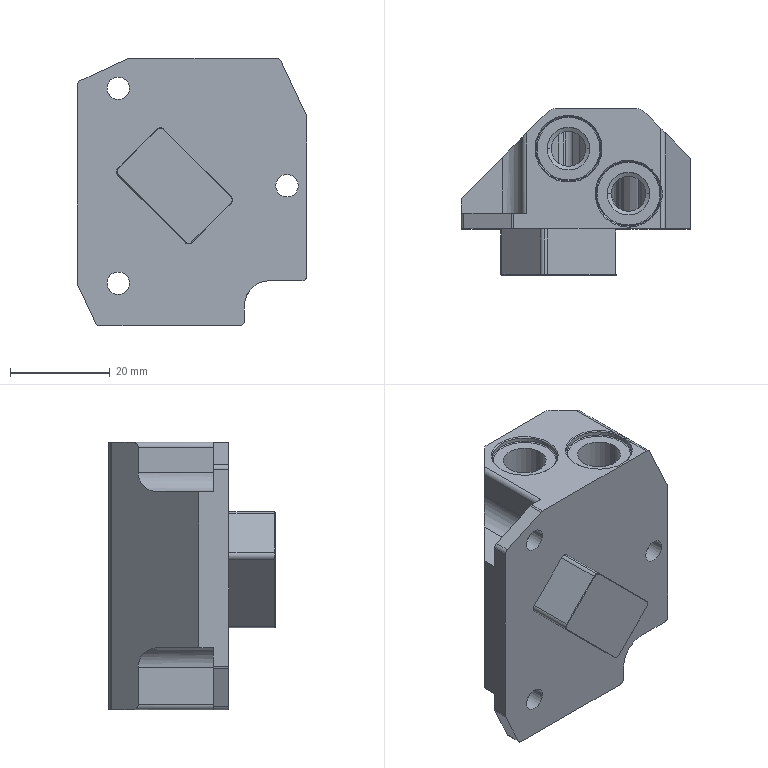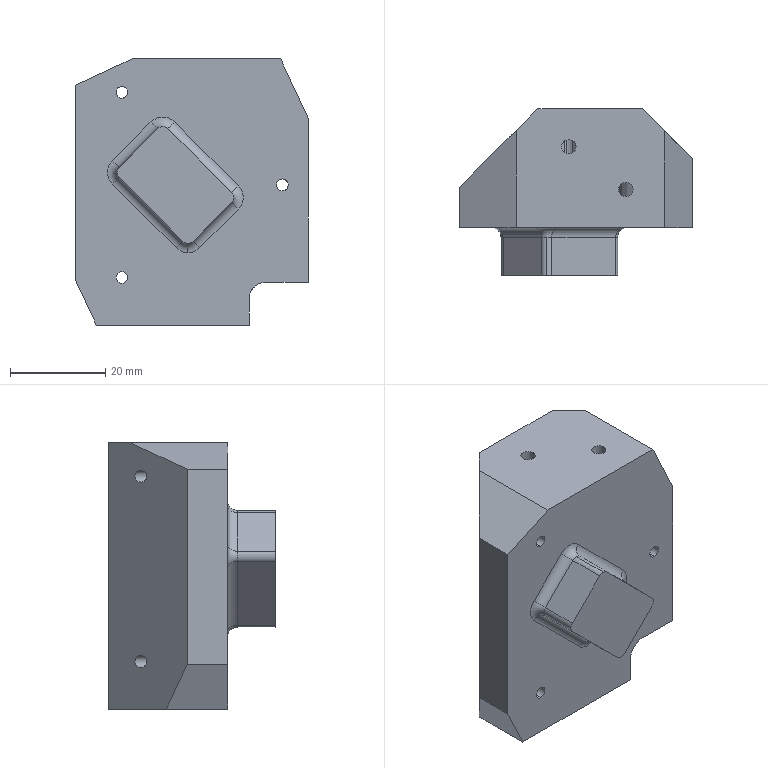CAM job | NX | 3+2 milling, 5-axis milling, drilling | part box 46 x 33.25 x 53.5 mm | stock box 49 x 35 x 56 mm
Tools:
number,name,description,diameter,corner_radius,flute_length,length,flutes
10,D3R0.2,Milling Tool-5 Parameters,3.0,0.2,50.0,75.0,2
0,D6R0.5,Milling Tool-5 Parameters,6.0,0.5,50.0,75.0,2
7,D3-9-D4-50-3T-ROUGH,D3-9-D4-50-3T,3.0,0.2,9.0,10.0,3
3,D5-15-D6-50-3T-ROUGH,D5-15-D6-50-3T,5.0,0.0,15.0,16.0,3
2,D10-30-D10-75-3T-ROUGH,D10-30-D10-75-3T-粗,10.0,0.0,30.0,75.0,2
5,D10-30-D10-75-3T-FINISH,D10-30-D10-75-3T,10.0,0.0,30.0,75.0,3
0,D63面刀,D63面刀,63.0,0.0,30.0,30.0,4
8,倒角D4-90度,倒角D4-90度,4.0,0.0,5.0,50.0,2
6,球刀R2-8-D4-50,球刀R2-8-D4-50,4.0,2.0,8.0,50.0,2
9,G8-1,Thread Mill,7.7,0.0,10.0,50.0,2
Operations:
program,operation,operation_type,tool,method,geometry_group,spindle_rpm,surface_speed,feed_per_tooth,feed_cut,feed_plunge,cut_length_mm,path_length_mm,cut_time_min,machine_time_min
NONE,PLANAR_MILL_6,PlanarMilling,D3-9-D4-50-3T-ROUGH,METHOD,C-G56,4500.0,70.0,0.0222,300.0,100.0,533.407,618.291,1.778,1.786
NONE,PLANAR_MILL_6_COPY,PlanarMilling,D3-9-D4-50-3T-ROUGH,METHOD,C-G56,4500.0,70.0,0.0222,300.0,100.0,93.82,186.111,0.3127,0.322
A1,PLANAR_MILL,PlanarMilling,D63面刀,METHOD,A-G54,3500.0,549.0,0.0571,800.0,100.0,126.5,182.5,0.1581,0.1637
A2,动态粗,CavityMilling,D10-30-D10-75-3T-ROUGH,METHOD,WORKPIECE_54,5500.0,172.0,0.1364,1500.0,100.0,5347.991,8574.346,3.44,3.763
A2,动态粗_COPY,CavityMilling,D5-15-D6-50-3T-ROUGH,METHOD,WORKPIECE_54,5500.0,86.0,0.0909,1500.0,100.0,1437.357,2628.154,0.9386,1.058
A3,CURVE_DRIVE,SurfaceContour,D6R0.5,METHOD,A-G54,5500.0,103.0,0.2727,3000.0,100.0,31035.578,31231.563,10.345,10.365
A4,PLANAR_MILL_1,PlanarMilling,D10-30-D10-75-3T-FINISH,METHOD,A-G54,4000.0,100.0,0.1178,800.0,100.0,453.139,559.139,0.5664,0.577
A4,PLANAR_MILL_2_COPY_1,PlanarMilling,D5-15-D6-50-3T-ROUGH,METHOD,A-G54,4500.0,70.0,0.0593,800.0,100.0,592.101,1419.752,0.7401,0.8229
A4,PLANAR_MILL_2,PlanarMilling,D5-15-D6-50-3T-ROUGH,METHOD,A-G54,4500.0,70.0,0.0593,800.0,100.0,190.71,630.914,0.2384,0.2824
A4,PLANAR_MILL_2_COPY,PlanarMilling,D5-15-D6-50-3T-ROUGH,METHOD,A-G54,4500.0,70.0,0.0593,800.0,100.0,288.693,485.736,0.3609,0.3806
A5,3_AXIS_DEBURRING,TpMultiAxisDeburring,球刀R2-8-D4-50,METHOD,A-G54,3500.0,43.0,0.1143,800.0,90.0,298.577,728.612,0.3745,0.3745
A6,PLANAR_MILL_COPY,PlanarMilling,D63面刀,METHOD,A-G54,3500.0,692.0,0.0286,400.0,100.0,126.5,182.52,0.3163,0.3219
B1,FLOOR_FACING,VolumeBased25DMillingOperation,D10-30-D10-75-3T-ROUGH,METHOD,B-G55,3500.0,109.0,0.1429,1000.0,100.0,84.508,124.308,0.0845,0.0885
B1,PLANAR_MILL_5_COPY,PlanarMilling,D10-30-D10-75-3T-ROUGH,METHOD,B-G55,3500.0,109.0,0.1429,1000.0,100.0,560.846,594.846,0.5608,0.5642
B1,HOLE_MILLING,CylinderMilling,D3-9-D4-50-3T-ROUGH,METHOD,B-G55,3000.0,28.0,0.0444,400.0,100.0,257.302,464.245,0.6433,0.6639
B1,FLOOR_FACING_1,VolumeBased25DMillingOperation,D10-30-D10-75-3T-FINISH,METHOD,B-G55,3500.0,109.0,0.0571,600.0,100.0,80.24,120.24,0.1337,0.1377
B1,PLANAR_MILL_5,PlanarMilling,D10-30-D10-75-3T-FINISH,METHOD,B-G55,3500.0,109.0,0.0571,600.0,100.0,561.135,595.135,0.9352,0.9386
B1,PLANAR_MILL_3,PlanarMilling,D10-30-D10-75-3T-FINISH,METHOD,B-G55,3500.0,109.0,0.0571,600.0,100.0,107.982,162.472,0.18,0.1854
B1,PLANAR_MILL_3_COPY,PlanarMilling,倒角D4-90度,METHOD,B-G55,3500.0,43.0,0.1429,1000.0,100.0,85.96,124.95,0.086,0.0899
B1,PLANAR_MILL_3_COPY_COPY,PlanarMilling,倒角D4-90度,METHOD,B-G55,3500.0,43.0,0.1429,1000.0,100.0,204.182,243.172,0.2042,0.2081
B1,PLANAR_MILL_3_COPY_COPY_1,PlanarMilling,倒角D4-90度,METHOD,B-G55,3500.0,43.0,0.1429,1000.0,100.0,28.34,223.655,0.0283,0.0479
C1,PLANAR_MILL_7,PlanarMilling,D5-15-D6-50-3T-ROUGH,METHOD,C-G56,4500.0,70.0,0.0222,300.0,100.0,543.659,650.337,1.812,1.823
C1,PLANAR_MILL_7_COPY_1,PlanarMilling,D5-15-D6-50-3T-ROUGH,METHOD,C-G56,4500.0,70.0,0.0222,300.0,100.0,215.142,343.432,0.7171,0.73
C1,PLANAR_MILL_4,PlanarMilling,D3R0.2,METHOD,C-G56,4500.0,42.0,0.0667,600.0,100.0,545.494,630.942,0.9092,0.9177
C1,PLANAR_MILL_4_COPY,PlanarMilling,D3R0.2,METHOD,C-G56,4500.0,42.0,0.0667,300.0,100.0,89.226,182.033,0.2974,0.3067
C1,PLANAR_MILL_7_COPY_COPY,PlanarMilling,倒角D4-90度,METHOD,C-G56,3000.0,37.0,0.1667,500.0,100.0,85.095,169.585,0.1702,0.1786
C1,PLANAR_MILL_7_COPY,PlanarMilling,倒角D4-90度,METHOD,C-G56,3000.0,37.0,0.1667,500.0,100.0,56.461,155.34,0.1129,0.1228
C1,THREAD_MILLING,ThreadMilling,G8-1,METHOD,C-G56,4000.0,96.0,0.0125,100.0,100.0,107.052,246.052,1.071,1.084